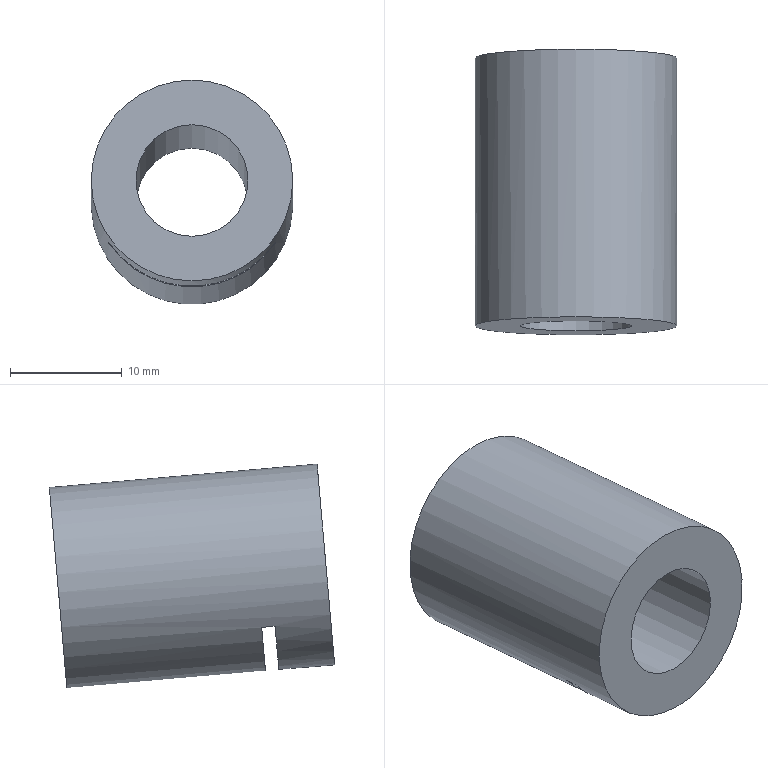Part | NX | features solid 2 | 1 solid | 7 faces | box 18 x 25.477 x 20.023 mm | volume 4174 mm3 | plane 5 | cylinder 2 | commonest cylinder face diameters 10 x1 18 x1
STEP:
#1=CARTESIAN_POINT('',(-561.105,-88.03,-33.124));
#2=VERTEX_POINT('',#1);
#3=CARTESIAN_POINT('',(-561.105,-88.814,-42.089));
#4=DIRECTION('',(0.,0.9962,-0.08716));
#5=DIRECTION('',(0.,0.08716,0.9962));
#6=AXIS2_PLACEMENT_3D('',#3,#4,#5);
#7=CIRCLE('',#6,9.);
#8=EDGE_CURVE('',#2,#2,#7,.F.);
#9=ORIENTED_EDGE('',*,*,#8,.F.);
#10=EDGE_LOOP('',(#9));
#11=FACE_BOUND('',#10,.T.);
#12=CARTESIAN_POINT('',(-561.105,-88.378,-37.108));
#13=VERTEX_POINT('',#12);
#14=CARTESIAN_POINT('',(-561.105,-88.814,-42.089));
#15=DIRECTION('',(0.,0.9962,-0.08716));
#16=DIRECTION('',(0.,0.08716,0.9962));
#17=AXIS2_PLACEMENT_3D('',#14,#15,#16);
#18=CIRCLE('',#17,5.);
#19=EDGE_CURVE('',#13,#13,#18,.F.);
#20=ORIENTED_EDGE('',*,*,#19,.T.);
#21=EDGE_LOOP('',(#20));
#22=FACE_BOUND('',#21,.T.);
#23=CARTESIAN_POINT('',(-561.105,-88.814,-42.089));
#24=DIRECTION('',(0.,0.9962,-0.08716));
#25=DIRECTION('',(-1.,0.,0.));
#26=AXIS2_PLACEMENT_3D('',#23,#24,#25);
#27=PLANE('',#26);
#28=ADVANCED_FACE('',(#11,#22),#27,.T.);
#29=CARTESIAN_POINT('',(-568.521,-108.186,-45.514));
#30=VERTEX_POINT('',#29);
#31=CARTESIAN_POINT('',(-568.521,-106.991,-45.619));
#32=VERTEX_POINT('',#31);
#33=CARTESIAN_POINT('',(-568.521,-54.591,-50.203));
#34=DIRECTION('',(0.,-0.9962,0.08716));
#35=VECTOR('',#34,1000.);
#36=LINE('',#33,#35);
#37=EDGE_CURVE('',#30,#32,#36,.F.);
#38=ORIENTED_EDGE('',*,*,#37,.F.);
#39=CARTESIAN_POINT('',(-553.69,-108.186,-45.514));
#40=VERTEX_POINT('',#39);
#41=CARTESIAN_POINT('',(-561.105,-107.742,-40.433));
#42=DIRECTION('',(0.,-0.9962,0.08716));
#43=DIRECTION('',(0.,-0.08716,-0.9962));
#44=AXIS2_PLACEMENT_3D('',#41,#42,#43);
#45=CIRCLE('',#44,9.);
#46=EDGE_CURVE('',#40,#30,#45,.F.);
#47=ORIENTED_EDGE('',*,*,#46,.F.);
#48=CARTESIAN_POINT('',(-553.69,-106.991,-45.619));
#49=VERTEX_POINT('',#48);
#50=CARTESIAN_POINT('',(-553.69,-54.591,-50.203));
#51=DIRECTION('',(0.,-0.9962,0.08716));
#52=VECTOR('',#51,1000.);
#53=LINE('',#50,#52);
#54=EDGE_CURVE('',#49,#40,#53,.T.);
#55=ORIENTED_EDGE('',*,*,#54,.F.);
#56=CARTESIAN_POINT('',(-561.105,-106.546,-40.538));
#57=DIRECTION('',(0.,-0.9962,0.08716));
#58=DIRECTION('',(0.,-0.08716,-0.9962));
#59=AXIS2_PLACEMENT_3D('',#56,#57,#58);
#60=CIRCLE('',#59,9.);
#61=EDGE_CURVE('',#49,#32,#60,.F.);
#62=ORIENTED_EDGE('',*,*,#61,.T.);
#63=EDGE_LOOP('',(#38,#47,#55,#62));
#64=FACE_BOUND('',#63,.T.);
#65=ORIENTED_EDGE('',*,*,#8,.T.);
#66=EDGE_LOOP('',(#65));
#67=FACE_BOUND('',#66,.T.);
#68=CARTESIAN_POINT('',(-561.105,-113.507,-48.963));
#69=VERTEX_POINT('',#68);
#70=CARTESIAN_POINT('',(-561.105,-112.723,-39.998));
#71=DIRECTION('',(0.,-0.9962,0.08716));
#72=DIRECTION('',(0.,-0.08716,-0.9962));
#73=AXIS2_PLACEMENT_3D('',#70,#71,#72);
#74=CIRCLE('',#73,9.);
#75=EDGE_CURVE('',#69,#69,#74,.F.);
#76=ORIENTED_EDGE('',*,*,#75,.T.);
#77=EDGE_LOOP('',(#76));
#78=FACE_BOUND('',#77,.T.);
#79=CARTESIAN_POINT('',(-561.105,-54.147,-45.122));
#80=DIRECTION('',(0.,-0.9962,0.08716));
#81=DIRECTION('',(1.,0.,0.));
#82=AXIS2_PLACEMENT_3D('',#79,#80,#81);
#83=CYLINDRICAL_SURFACE('',#82,9.);
#84=ADVANCED_FACE('',(#64,#67,#78),#83,.T.);
#85=CARTESIAN_POINT('',(-561.105,-113.159,-44.979));
#86=VERTEX_POINT('',#85);
#87=CARTESIAN_POINT('',(-561.105,-112.723,-39.998));
#88=DIRECTION('',(0.,-0.9962,0.08716));
#89=DIRECTION('',(0.,-0.08716,-0.9962));
#90=AXIS2_PLACEMENT_3D('',#87,#88,#89);
#91=CIRCLE('',#90,5.);
#92=EDGE_CURVE('',#86,#86,#91,.F.);
#93=ORIENTED_EDGE('',*,*,#92,.T.);
#94=EDGE_LOOP('',(#93));
#95=FACE_BOUND('',#94,.T.);
#96=ORIENTED_EDGE('',*,*,#75,.F.);
#97=EDGE_LOOP('',(#96));
#98=FACE_BOUND('',#97,.T.);
#99=CARTESIAN_POINT('',(-561.105,-112.723,-39.998));
#100=DIRECTION('',(0.,-0.9962,0.08716));
#101=DIRECTION('',(-1.,0.,0.));
#102=AXIS2_PLACEMENT_3D('',#99,#100,#101);
#103=PLANE('',#102);
#104=ADVANCED_FACE('',(#95,#98),#103,.T.);
#105=ORIENTED_EDGE('',*,*,#19,.F.);
#106=EDGE_LOOP('',(#105));
#107=FACE_BOUND('',#106,.T.);
#108=ORIENTED_EDGE('',*,*,#92,.F.);
#109=EDGE_LOOP('',(#108));
#110=FACE_BOUND('',#109,.T.);
#111=CARTESIAN_POINT('',(-561.105,-107.941,-40.416));
#112=DIRECTION('',(0.,0.9962,-0.08716));
#113=DIRECTION('',(-1.,0.,0.));
#114=AXIS2_PLACEMENT_3D('',#111,#112,#113);
#115=CYLINDRICAL_SURFACE('',#114,5.);
#116=ADVANCED_FACE('',(#107,#110),#115,.F.);
#117=CARTESIAN_POINT('',(-568.589,-106.991,-45.619));
#118=DIRECTION('',(-1.,0.,0.));
#119=VECTOR('',#118,1000.);
#120=LINE('',#117,#119);
#121=EDGE_CURVE('',#32,#49,#120,.F.);
#122=ORIENTED_EDGE('',*,*,#121,.F.);
#123=ORIENTED_EDGE('',*,*,#61,.F.);
#124=EDGE_LOOP('',(#122,#123));
#125=FACE_BOUND('',#124,.T.);
#126=CARTESIAN_POINT('',(-568.589,-111.349,-95.428));
#127=DIRECTION('',(0.,-0.9962,0.08716));
#128=DIRECTION('',(0.,-0.08716,-0.9962));
#129=AXIS2_PLACEMENT_3D('',#126,#127,#128);
#130=PLANE('',#129);
#131=ADVANCED_FACE('',(#125),#130,.T.);
#132=ORIENTED_EDGE('',*,*,#46,.T.);
#133=CARTESIAN_POINT('',(-568.589,-108.186,-45.514));
#134=DIRECTION('',(-1.,0.,0.));
#135=VECTOR('',#134,1000.);
#136=LINE('',#133,#135);
#137=EDGE_CURVE('',#30,#40,#136,.F.);
#138=ORIENTED_EDGE('',*,*,#137,.T.);
#139=EDGE_LOOP('',(#132,#138));
#140=FACE_BOUND('',#139,.T.);
#141=CARTESIAN_POINT('',(-568.589,-112.544,-95.324));
#142=DIRECTION('',(0.,-0.9962,0.08716));
#143=DIRECTION('',(0.,-0.08716,-0.9962));
#144=AXIS2_PLACEMENT_3D('',#141,#142,#143);
#145=PLANE('',#144);
#146=ADVANCED_FACE('',(#140),#145,.F.);
#147=ORIENTED_EDGE('',*,*,#37,.T.);
#148=ORIENTED_EDGE('',*,*,#121,.T.);
#149=ORIENTED_EDGE('',*,*,#54,.T.);
#150=ORIENTED_EDGE('',*,*,#137,.F.);
#151=EDGE_LOOP('',(#147,#148,#149,#150));
#152=FACE_BOUND('',#151,.T.);
#153=CARTESIAN_POINT('',(-568.589,-108.186,-45.514));
#154=DIRECTION('',(0.,0.08716,0.9962));
#155=DIRECTION('',(0.,0.9962,-0.08716));
#156=AXIS2_PLACEMENT_3D('',#153,#154,#155);
#157=PLANE('',#156);
#158=ADVANCED_FACE('',(#152),#157,.F.);
#159=CLOSED_SHELL('',(#28,#84,#104,#116,#131,#146,#158));
#160=MANIFOLD_SOLID_BREP('',#159);
#161=(LENGTH_UNIT()NAMED_UNIT(*)SI_UNIT(.MILLI.,.METRE.));
#162=UNCERTAINTY_MEASURE_WITH_UNIT(LENGTH_MEASURE(0.00001),#161,'','');
#163=(NAMED_UNIT(*)PLANE_ANGLE_UNIT()SI_UNIT($,.RADIAN.));
#164=(NAMED_UNIT(*)SI_UNIT($,.STERADIAN.)SOLID_ANGLE_UNIT());
#165=(GEOMETRIC_REPRESENTATION_CONTEXT(3)GLOBAL_UNCERTAINTY_ASSIGNED_CONTEXT((#162))GLOBAL_UNIT_ASSIGNED_CONTEXT((#161,#163,#164))REPRESENTATION_CONTEXT('',''));
#166=ADVANCED_BREP_SHAPE_REPRESENTATION('',(#160),#165);